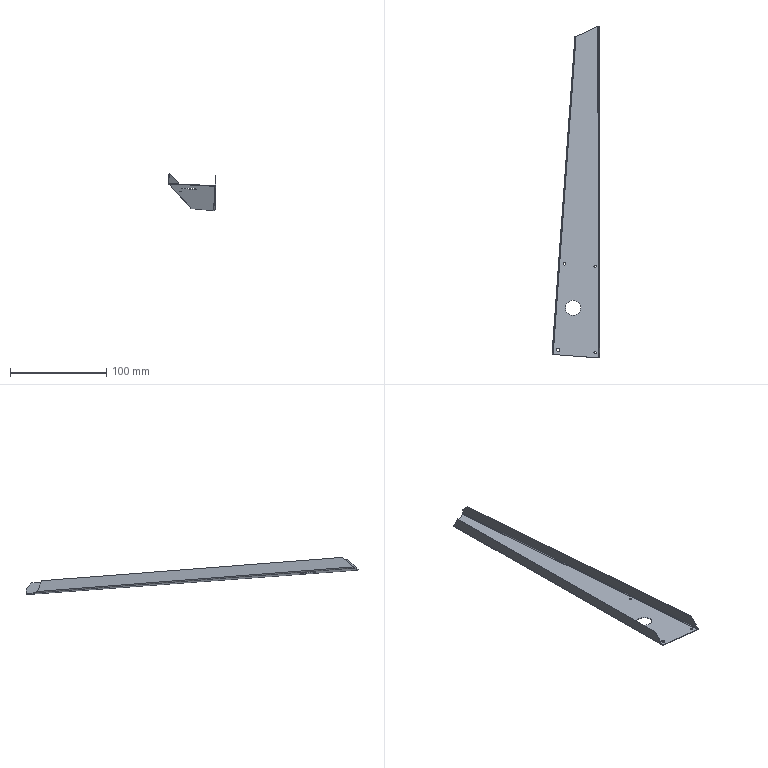Part | SolidWorks | features BaseBody 1 | 1 solid | 37 faces | box 49.869 x 345.626 x 38.793 mm | volume 9891 mm3 | cylinder 16 | plane 15 | spline 6 | commonest cylinder face diameters 2.4 x6 1.473 x3 2.473 x3 3.385 x2 15.9 x2
STEP:
#1=CARTESIAN_POINT('',(-25.934,44.235,46.553));
#2=VERTEX_POINT('',#1);
#3=CARTESIAN_POINT('',(-25.934,60.092,45.382));
#4=VERTEX_POINT('',#3);
#5=CARTESIAN_POINT('',(-25.934,52.163,45.968));
#6=DIRECTION('',(-0.05227,-0.07356,-0.9959));
#7=DIRECTION('',(0.,-0.9973,0.07366));
#8=AXIS2_PLACEMENT_3D('',#5,#6,#7);
#9=CIRCLE('',#8,7.95);
#10=EDGE_CURVE('',#2,#4,#9,.T.);
#11=ORIENTED_EDGE('',*,*,#10,.T.);
#12=CARTESIAN_POINT('',(-25.908,60.128,45.88));
#13=VERTEX_POINT('',#12);
#14=CARTESIAN_POINT('',(-25.934,60.092,45.382));
#15=DIRECTION('',(0.05227,0.07356,0.9959));
#16=VECTOR('',#15,1000.);
#17=LINE('',#14,#16);
#18=EDGE_CURVE('',#4,#13,#17,.T.);
#19=ORIENTED_EDGE('',*,*,#18,.T.);
#20=CARTESIAN_POINT('',(-25.908,44.272,47.051));
#21=VERTEX_POINT('',#20);
#22=CARTESIAN_POINT('',(-25.908,52.2,46.466));
#23=DIRECTION('',(0.05227,0.07356,0.9959));
#24=DIRECTION('',(0.,-0.9973,0.07366));
#25=AXIS2_PLACEMENT_3D('',#22,#23,#24);
#26=CIRCLE('',#25,7.95);
#27=EDGE_CURVE('',#13,#21,#26,.T.);
#28=ORIENTED_EDGE('',*,*,#27,.T.);
#29=CARTESIAN_POINT('',(-25.934,44.235,46.553));
#30=DIRECTION('',(0.05227,0.07356,0.9959));
#31=VECTOR('',#30,1000.);
#32=LINE('',#29,#31);
#33=EDGE_CURVE('',#2,#21,#32,.T.);
#34=ORIENTED_EDGE('',*,*,#33,.F.);
#35=EDGE_LOOP('',(#11,#19,#28,#34));
#36=FACE_OUTER_BOUND('',#35,.T.);
#37=CARTESIAN_POINT('',(-25.934,52.163,45.968));
#38=DIRECTION('',(0.05227,0.07356,0.9959));
#39=DIRECTION('',(0.,-0.9973,0.07366));
#40=AXIS2_PLACEMENT_3D('',#37,#38,#39);
#41=CYLINDRICAL_SURFACE('',#40,7.95);
#42=ADVANCED_FACE('',(#36),#41,.F.);
#43=CARTESIAN_POINT('',(-3.009,96.582,41.484));
#44=VERTEX_POINT('',#43);
#45=CARTESIAN_POINT('',(-3.009,94.189,41.661));
#46=VERTEX_POINT('',#45);
#47=CARTESIAN_POINT('',(-3.009,95.385,41.572));
#48=DIRECTION('',(0.05227,0.07356,0.9959));
#49=DIRECTION('',(0.,-0.9973,0.07366));
#50=AXIS2_PLACEMENT_3D('',#47,#48,#49);
#51=CIRCLE('',#50,1.2);
#52=EDGE_CURVE('',#44,#46,#51,.T.);
#53=ORIENTED_EDGE('',*,*,#52,.F.);
#54=CARTESIAN_POINT('',(-2.982,96.619,41.982));
#55=VERTEX_POINT('',#54);
#56=CARTESIAN_POINT('',(-3.009,96.582,41.484));
#57=DIRECTION('',(0.05227,0.07356,0.9959));
#58=VECTOR('',#57,1000.);
#59=LINE('',#56,#58);
#60=EDGE_CURVE('',#44,#55,#59,.T.);
#61=ORIENTED_EDGE('',*,*,#60,.T.);
#62=CARTESIAN_POINT('',(-2.982,94.225,42.159));
#63=VERTEX_POINT('',#62);
#64=CARTESIAN_POINT('',(-2.982,95.422,42.07));
#65=DIRECTION('',(0.05227,0.07356,0.9959));
#66=DIRECTION('',(0.,-0.9973,0.07366));
#67=AXIS2_PLACEMENT_3D('',#64,#65,#66);
#68=CIRCLE('',#67,1.2);
#69=EDGE_CURVE('',#55,#63,#68,.T.);
#70=ORIENTED_EDGE('',*,*,#69,.T.);
#71=CARTESIAN_POINT('',(-3.009,94.189,41.661));
#72=DIRECTION('',(0.05227,0.07356,0.9959));
#73=VECTOR('',#72,1000.);
#74=LINE('',#71,#73);
#75=EDGE_CURVE('',#46,#63,#74,.T.);
#76=ORIENTED_EDGE('',*,*,#75,.F.);
#77=EDGE_LOOP('',(#53,#61,#70,#76));
#78=FACE_OUTER_BOUND('',#77,.T.);
#79=CARTESIAN_POINT('',(-3.009,95.385,41.572));
#80=DIRECTION('',(0.05227,0.07356,0.9959));
#81=DIRECTION('',(0.,-0.9973,0.07366));
#82=AXIS2_PLACEMENT_3D('',#79,#80,#81);
#83=CYLINDRICAL_SURFACE('',#82,1.2);
#84=ADVANCED_FACE('',(#78),#83,.F.);
#85=CARTESIAN_POINT('',(-34.851,99.051,42.973));
#86=VERTEX_POINT('',#85);
#87=CARTESIAN_POINT('',(-34.851,96.658,43.149));
#88=VERTEX_POINT('',#87);
#89=CARTESIAN_POINT('',(-34.851,97.854,43.061));
#90=DIRECTION('',(0.05227,0.07356,0.9959));
#91=DIRECTION('',(0.,-0.9973,0.07366));
#92=AXIS2_PLACEMENT_3D('',#89,#90,#91);
#93=CIRCLE('',#92,1.2);
#94=EDGE_CURVE('',#86,#88,#93,.T.);
#95=ORIENTED_EDGE('',*,*,#94,.F.);
#96=CARTESIAN_POINT('',(-34.825,99.088,43.471));
#97=VERTEX_POINT('',#96);
#98=CARTESIAN_POINT('',(-34.851,99.051,42.973));
#99=DIRECTION('',(0.05227,0.07356,0.9959));
#100=VECTOR('',#99,1000.);
#101=LINE('',#98,#100);
#102=EDGE_CURVE('',#86,#97,#101,.T.);
#103=ORIENTED_EDGE('',*,*,#102,.T.);
#104=CARTESIAN_POINT('',(-34.825,96.694,43.647));
#105=VERTEX_POINT('',#104);
#106=CARTESIAN_POINT('',(-34.825,97.891,43.559));
#107=DIRECTION('',(0.05227,0.07356,0.9959));
#108=DIRECTION('',(0.,-0.9973,0.07366));
#109=AXIS2_PLACEMENT_3D('',#106,#107,#108);
#110=CIRCLE('',#109,1.2);
#111=EDGE_CURVE('',#97,#105,#110,.T.);
#112=ORIENTED_EDGE('',*,*,#111,.T.);
#113=CARTESIAN_POINT('',(-34.851,96.658,43.149));
#114=DIRECTION('',(0.05227,0.07356,0.9959));
#115=VECTOR('',#114,1000.);
#116=LINE('',#113,#115);
#117=EDGE_CURVE('',#88,#105,#116,.T.);
#118=ORIENTED_EDGE('',*,*,#117,.F.);
#119=EDGE_LOOP('',(#95,#103,#112,#118));
#120=FACE_OUTER_BOUND('',#119,.T.);
#121=CARTESIAN_POINT('',(-34.851,97.854,43.061));
#122=DIRECTION('',(0.05227,0.07356,0.9959));
#123=DIRECTION('',(0.,-0.9973,0.07366));
#124=AXIS2_PLACEMENT_3D('',#121,#122,#123);
#125=CYLINDRICAL_SURFACE('',#124,1.2);
#126=ADVANCED_FACE('',(#120),#125,.F.);
#127=CARTESIAN_POINT('',(-3.008,6.583,48.131));
#128=VERTEX_POINT('',#127);
#129=CARTESIAN_POINT('',(-3.008,4.189,48.308));
#130=VERTEX_POINT('',#129);
#131=CARTESIAN_POINT('',(-3.008,5.386,48.22));
#132=DIRECTION('',(0.05227,0.07356,0.9959));
#133=DIRECTION('',(0.,-0.9973,0.07366));
#134=AXIS2_PLACEMENT_3D('',#131,#132,#133);
#135=CIRCLE('',#134,1.2);
#136=EDGE_CURVE('',#128,#130,#135,.T.);
#137=ORIENTED_EDGE('',*,*,#136,.F.);
#138=CARTESIAN_POINT('',(-2.982,6.619,48.629));
#139=VERTEX_POINT('',#138);
#140=CARTESIAN_POINT('',(-3.008,6.583,48.131));
#141=DIRECTION('',(0.05227,0.07356,0.9959));
#142=VECTOR('',#141,1000.);
#143=LINE('',#140,#142);
#144=EDGE_CURVE('',#128,#139,#143,.T.);
#145=ORIENTED_EDGE('',*,*,#144,.T.);
#146=CARTESIAN_POINT('',(-2.982,4.226,48.806));
#147=VERTEX_POINT('',#146);
#148=CARTESIAN_POINT('',(-2.982,5.423,48.718));
#149=DIRECTION('',(0.05227,0.07356,0.9959));
#150=DIRECTION('',(0.,-0.9973,0.07366));
#151=AXIS2_PLACEMENT_3D('',#148,#149,#150);
#152=CIRCLE('',#151,1.2);
#153=EDGE_CURVE('',#139,#147,#152,.T.);
#154=ORIENTED_EDGE('',*,*,#153,.T.);
#155=CARTESIAN_POINT('',(-3.008,4.189,48.308));
#156=DIRECTION('',(0.05227,0.07356,0.9959));
#157=VECTOR('',#156,1000.);
#158=LINE('',#155,#157);
#159=EDGE_CURVE('',#130,#147,#158,.T.);
#160=ORIENTED_EDGE('',*,*,#159,.F.);
#161=EDGE_LOOP('',(#137,#145,#154,#160));
#162=FACE_OUTER_BOUND('',#161,.T.);
#163=CARTESIAN_POINT('',(-3.008,5.386,48.22));
#164=DIRECTION('',(0.05227,0.07356,0.9959));
#165=DIRECTION('',(0.,-0.9973,0.07366));
#166=AXIS2_PLACEMENT_3D('',#163,#164,#165);
#167=CYLINDRICAL_SURFACE('',#166,1.2);
#168=ADVANCED_FACE('',(#162),#167,.F.);
#169=CARTESIAN_POINT('',(-41.464,10.056,49.893));
#170=VERTEX_POINT('',#169);
#171=CARTESIAN_POINT('',(-41.464,6.68,50.142));
#172=VERTEX_POINT('',#171);
#173=CARTESIAN_POINT('',(-41.464,8.368,50.018));
#174=DIRECTION('',(0.05227,0.07356,0.9959));
#175=DIRECTION('',(0.,-0.9973,0.07366));
#176=AXIS2_PLACEMENT_3D('',#173,#174,#175);
#177=CIRCLE('',#176,1.693);
#178=EDGE_CURVE('',#170,#172,#177,.T.);
#179=ORIENTED_EDGE('',*,*,#178,.F.);
#180=CARTESIAN_POINT('',(-41.438,10.092,50.391));
#181=VERTEX_POINT('',#180);
#182=CARTESIAN_POINT('',(-41.464,10.056,49.893));
#183=DIRECTION('',(0.05227,0.07356,0.9959));
#184=VECTOR('',#183,1000.);
#185=LINE('',#182,#184);
#186=EDGE_CURVE('',#170,#181,#185,.T.);
#187=ORIENTED_EDGE('',*,*,#186,.T.);
#188=CARTESIAN_POINT('',(-41.438,6.716,50.64));
#189=VERTEX_POINT('',#188);
#190=CARTESIAN_POINT('',(-41.438,8.404,50.516));
#191=DIRECTION('',(0.05227,0.07356,0.9959));
#192=DIRECTION('',(0.,-0.9973,0.07366));
#193=AXIS2_PLACEMENT_3D('',#190,#191,#192);
#194=CIRCLE('',#193,1.693);
#195=EDGE_CURVE('',#181,#189,#194,.T.);
#196=ORIENTED_EDGE('',*,*,#195,.T.);
#197=CARTESIAN_POINT('',(-41.464,6.68,50.142));
#198=DIRECTION('',(0.05227,0.07356,0.9959));
#199=VECTOR('',#198,1000.);
#200=LINE('',#197,#199);
#201=EDGE_CURVE('',#172,#189,#200,.T.);
#202=ORIENTED_EDGE('',*,*,#201,.F.);
#203=EDGE_LOOP('',(#179,#187,#196,#202));
#204=FACE_OUTER_BOUND('',#203,.T.);
#205=CARTESIAN_POINT('',(-41.464,8.368,50.018));
#206=DIRECTION('',(0.05227,0.07356,0.9959));
#207=DIRECTION('',(0.,-0.9973,0.07366));
#208=AXIS2_PLACEMENT_3D('',#205,#206,#207);
#209=CYLINDRICAL_SURFACE('',#208,1.693);
#210=ADVANCED_FACE('',(#204),#209,.F.);
#211=CARTESIAN_POINT('',(0.4134,345.618,23.653));
#212=VERTEX_POINT('',#211);
#213=CARTESIAN_POINT('',(-0.1031,345.249,23.468));
#214=VERTEX_POINT('',#213);
#215=CARTESIAN_POINT('',(0.4134,345.618,23.653));
#216=CARTESIAN_POINT('',(0.345,345.554,23.59));
#217=CARTESIAN_POINT('',(0.2656,345.492,23.542));
#218=CARTESIAN_POINT('',(0.08824,345.368,23.478));
#219=CARTESIAN_POINT('',(-0.007361,345.308,23.463));
#220=CARTESIAN_POINT('',(-0.1031,345.249,23.468));
#221=B_SPLINE_CURVE_WITH_KNOTS('',3,(#215,#216,#217,#218,#219,#220),.UNSPECIFIED.,.F.,.F.,(4,2,4),(0.,0.0003341,0.0006683),.UNSPECIFIED.);
#222=EDGE_CURVE('',#212,#214,#221,.T.);
#223=ORIENTED_EDGE('',*,*,#222,.T.);
#224=CARTESIAN_POINT('',(0.5636,0.05796,48.929));
#225=VERTEX_POINT('',#224);
#226=CARTESIAN_POINT('',(-0.1078,347.675,23.289));
#227=DIRECTION('',(0.001926,-0.9973,0.07356));
#228=VECTOR('',#227,1000.);
#229=LINE('',#226,#228);
#230=EDGE_CURVE('',#214,#225,#229,.T.);
#231=ORIENTED_EDGE('',*,*,#230,.T.);
#232=CARTESIAN_POINT('',(1.081,0.01805,49.144));
#233=VERTEX_POINT('',#232);
#234=CARTESIAN_POINT('',(0.5636,0.05796,48.929));
#235=CARTESIAN_POINT('',(0.7548,0.03949,48.93));
#236=CARTESIAN_POINT('',(0.9448,0.02675,49.009));
#237=CARTESIAN_POINT('',(1.081,0.01805,49.144));
#238=B_SPLINE_CURVE_WITH_KNOTS('',3,(#234,#235,#236,#237),.UNSPECIFIED.,.F.,.F.,(4,4),(0.06296,1.),.UNSPECIFIED.);
#239=EDGE_CURVE('',#225,#233,#238,.T.);
#240=ORIENTED_EDGE('',*,*,#239,.T.);
#241=CARTESIAN_POINT('',(1.299,0.7061,49.6));
#242=VERTEX_POINT('',#241);
#243=CARTESIAN_POINT('',(1.081,0.01805,49.144));
#244=CARTESIAN_POINT('',(1.215,0.2454,49.26));
#245=CARTESIAN_POINT('',(1.294,0.4748,49.428));
#246=CARTESIAN_POINT('',(1.299,0.7061,49.6));
#247=B_SPLINE_CURVE_WITH_KNOTS('',3,(#243,#244,#245,#246),.UNSPECIFIED.,.F.,.F.,(4,4),(0.,0.0008625),.UNSPECIFIED.);
#248=EDGE_CURVE('',#233,#242,#247,.T.);
#249=ORIENTED_EDGE('',*,*,#248,.T.);
#250=CARTESIAN_POINT('',(0.6327,345.6,24.161));
#251=VERTEX_POINT('',#250);
#252=CARTESIAN_POINT('',(0.9663,172.856,36.903));
#253=DIRECTION('',(-0.001926,0.9973,-0.07356));
#254=VECTOR('',#253,1000.);
#255=LINE('',#252,#254);
#256=EDGE_CURVE('',#242,#251,#255,.T.);
#257=ORIENTED_EDGE('',*,*,#256,.T.);
#258=CARTESIAN_POINT('',(0.6327,345.6,24.161));
#259=CARTESIAN_POINT('',(0.6277,345.605,23.972));
#260=CARTESIAN_POINT('',(0.5474,345.609,23.786));
#261=CARTESIAN_POINT('',(0.4134,345.618,23.653));
#262=B_SPLINE_CURVE_WITH_KNOTS('',3,(#258,#259,#260,#261),.UNSPECIFIED.,.F.,.F.,(4,4),(0.,1.),.UNSPECIFIED.);
#263=EDGE_CURVE('',#251,#212,#262,.T.);
#264=ORIENTED_EDGE('',*,*,#263,.T.);
#265=EDGE_LOOP('',(#223,#231,#240,#249,#257,#264));
#266=FACE_OUTER_BOUND('',#265,.T.);
#267=CARTESIAN_POINT('',(-0.1078,347.729,24.023));
#268=DIRECTION('',(0.001926,-0.9973,0.07356));
#269=DIRECTION('',(0.,-0.07356,-0.9973));
#270=AXIS2_PLACEMENT_3D('',#267,#268,#269);
#271=CYLINDRICAL_SURFACE('',#270,0.7366);
#272=ADVANCED_FACE('',(#266),#271,.F.);
#273=CARTESIAN_POINT('',(-0.1031,345.212,22.969));
#274=VERTEX_POINT('',#273);
#275=CARTESIAN_POINT('',(-0.1677,345.188,22.973));
#276=VERTEX_POINT('',#275);
#277=CARTESIAN_POINT('',(-0.1031,345.212,22.969));
#278=CARTESIAN_POINT('',(-0.1246,345.204,22.97));
#279=CARTESIAN_POINT('',(-0.1461,345.196,22.971));
#280=CARTESIAN_POINT('',(-0.1677,345.188,22.973));
#281=B_SPLINE_CURVE_WITH_KNOTS('',3,(#277,#278,#279,#280),.UNSPECIFIED.,.F.,.F.,(4,4),(0.00102,0.001088),.UNSPECIFIED.);
#282=EDGE_CURVE('',#274,#276,#281,.T.);
#283=ORIENTED_EDGE('',*,*,#282,.F.);
#284=CARTESIAN_POINT('',(0.5636,0.02118,48.43));
#285=VERTEX_POINT('',#284);
#286=CARTESIAN_POINT('',(-0.1078,347.638,22.79));
#287=DIRECTION('',(0.001926,-0.9973,0.07356));
#288=VECTOR('',#287,1000.);
#289=LINE('',#286,#288);
#290=EDGE_CURVE('',#274,#285,#289,.T.);
#291=ORIENTED_EDGE('',*,*,#290,.T.);
#292=CARTESIAN_POINT('',(0.499,0.02497,48.432));
#293=VERTEX_POINT('',#292);
#294=CARTESIAN_POINT('',(0.499,0.02497,48.432));
#295=CARTESIAN_POINT('',(0.5205,0.02367,48.431));
#296=CARTESIAN_POINT('',(0.5421,0.0224,48.43));
#297=CARTESIAN_POINT('',(0.5636,0.02118,48.43));
#298=B_SPLINE_CURVE_WITH_KNOTS('',3,(#294,#295,#296,#297),.UNSPECIFIED.,.F.,.F.,(4,4),(0.,0.06296),.UNSPECIFIED.);
#299=EDGE_CURVE('',#293,#285,#298,.T.);
#300=ORIENTED_EDGE('',*,*,#299,.F.);
#301=CARTESIAN_POINT('',(-0.1677,345.188,22.973));
#302=DIRECTION('',(0.001926,-0.9973,0.07356));
#303=VECTOR('',#302,1000.);
#304=LINE('',#301,#303);
#305=EDGE_CURVE('',#276,#293,#304,.T.);
#306=ORIENTED_EDGE('',*,*,#305,.F.);
#307=EDGE_LOOP('',(#283,#291,#300,#306));
#308=FACE_OUTER_BOUND('',#307,.T.);
#309=CARTESIAN_POINT('',(-0.1078,347.729,24.023));
#310=DIRECTION('',(0.001926,-0.9973,0.07356));
#311=DIRECTION('',(0.,-0.07356,-0.9973));
#312=AXIS2_PLACEMENT_3D('',#309,#310,#311);
#313=CYLINDRICAL_SURFACE('',#312,1.237);
#314=ADVANCED_FACE('',(#308),#313,.T.);
#315=ORIENTED_EDGE('',*,*,#18,.F.);
#316=CARTESIAN_POINT('',(-25.934,52.163,45.968));
#317=DIRECTION('',(-0.05227,-0.07356,-0.9959));
#318=DIRECTION('',(0.,-0.9973,0.07366));
#319=AXIS2_PLACEMENT_3D('',#316,#317,#318);
#320=CIRCLE('',#319,7.95);
#321=EDGE_CURVE('',#4,#2,#320,.T.);
#322=ORIENTED_EDGE('',*,*,#321,.T.);
#323=ORIENTED_EDGE('',*,*,#33,.T.);
#324=CARTESIAN_POINT('',(-25.908,52.2,46.466));
#325=DIRECTION('',(0.05227,0.07356,0.9959));
#326=DIRECTION('',(0.,-0.9973,0.07366));
#327=AXIS2_PLACEMENT_3D('',#324,#325,#326);
#328=CIRCLE('',#327,7.95);
#329=EDGE_CURVE('',#21,#13,#328,.T.);
#330=ORIENTED_EDGE('',*,*,#329,.T.);
#331=EDGE_LOOP('',(#315,#322,#323,#330));
#332=FACE_OUTER_BOUND('',#331,.T.);
#333=CARTESIAN_POINT('',(-25.934,52.163,45.968));
#334=DIRECTION('',(0.05227,0.07356,0.9959));
#335=DIRECTION('',(0.,-0.9973,0.07366));
#336=AXIS2_PLACEMENT_3D('',#333,#334,#335);
#337=CYLINDRICAL_SURFACE('',#336,7.95);
#338=ADVANCED_FACE('',(#332),#337,.F.);
#339=CARTESIAN_POINT('',(-2.982,95.422,42.07));
#340=DIRECTION('',(0.05227,0.07356,0.9959));
#341=DIRECTION('',(0.,-0.9973,0.07366));
#342=AXIS2_PLACEMENT_3D('',#339,#340,#341);
#343=CIRCLE('',#342,1.2);
#344=EDGE_CURVE('',#63,#55,#343,.T.);
#345=ORIENTED_EDGE('',*,*,#344,.F.);
#346=ORIENTED_EDGE('',*,*,#69,.F.);
#347=EDGE_LOOP('',(#345,#346));
#348=FACE_BOUND('',#347,.T.);
#349=CARTESIAN_POINT('',(-34.825,97.891,43.559));
#350=DIRECTION('',(0.05227,0.07356,0.9959));
#351=DIRECTION('',(0.,-0.9973,0.07366));
#352=AXIS2_PLACEMENT_3D('',#349,#350,#351);
#353=CIRCLE('',#352,1.2);
#354=EDGE_CURVE('',#105,#97,#353,.T.);
#355=ORIENTED_EDGE('',*,*,#354,.F.);
#356=ORIENTED_EDGE('',*,*,#111,.F.);
#357=EDGE_LOOP('',(#355,#356));
#358=FACE_BOUND('',#357,.T.);
#359=CARTESIAN_POINT('',(-2.982,5.423,48.718));
#360=DIRECTION('',(0.05227,0.07356,0.9959));
#361=DIRECTION('',(0.,-0.9973,0.07366));
#362=AXIS2_PLACEMENT_3D('',#359,#360,#361);
#363=CIRCLE('',#362,1.2);
#364=EDGE_CURVE('',#147,#139,#363,.T.);
#365=ORIENTED_EDGE('',*,*,#364,.F.);
#366=ORIENTED_EDGE('',*,*,#153,.F.);
#367=EDGE_LOOP('',(#365,#366));
#368=FACE_BOUND('',#367,.T.);
#369=CARTESIAN_POINT('',(-41.438,8.404,50.516));
#370=DIRECTION('',(0.05227,0.07356,0.9959));
#371=DIRECTION('',(0.,-0.9973,0.07366));
#372=AXIS2_PLACEMENT_3D('',#369,#370,#371);
#373=CIRCLE('',#372,1.693);
#374=EDGE_CURVE('',#189,#181,#373,.T.);
#375=ORIENTED_EDGE('',*,*,#374,.F.);
#376=ORIENTED_EDGE('',*,*,#195,.F.);
#377=EDGE_LOOP('',(#375,#376));
#378=FACE_BOUND('',#377,.T.);
#379=ORIENTED_EDGE('',*,*,#329,.F.);
#380=ORIENTED_EDGE('',*,*,#27,.F.);
#381=EDGE_LOOP('',(#379,#380));
#382=FACE_BOUND('',#381,.T.);
#383=CARTESIAN_POINT('',(-46.66,3.629,51.142));
#384=VERTEX_POINT('',#383);
#385=CARTESIAN_POINT('',(-22.827,334.825,25.429));
#386=VERTEX_POINT('',#385);
#387=CARTESIAN_POINT('',(-34.236,176.282,37.738));
#388=DIRECTION('',(0.07156,0.9944,-0.07721));
#389=VECTOR('',#388,1000.);
#390=LINE('',#387,#389);
#391=EDGE_CURVE('',#384,#386,#390,.T.);
#392=ORIENTED_EDGE('',*,*,#391,.F.);
#393=CARTESIAN_POINT('',(0.5251,0.06175,48.93));
#394=VERTEX_POINT('',#393);
#395=CARTESIAN_POINT('',(-22.926,1.835,50.029));
#396=DIRECTION('',(-0.9961,0.07531,0.04671));
#397=VECTOR('',#396,1000.);
#398=LINE('',#395,#397);
#399=EDGE_CURVE('',#394,#384,#398,.T.);
#400=ORIENTED_EDGE('',*,*,#399,.F.);
#401=CARTESIAN_POINT('',(-0.1415,345.225,23.47));
#402=VERTEX_POINT('',#401);
#403=CARTESIAN_POINT('',(-0.1463,347.675,23.29));
#404=DIRECTION('',(0.001926,-0.9973,0.07356));
#405=VECTOR('',#404,1000.);
#406=LINE('',#403,#405);
#407=EDGE_CURVE('',#402,#394,#406,.T.);
#408=ORIENTED_EDGE('',*,*,#407,.F.);
#409=CARTESIAN_POINT('',(-22.827,334.825,25.429));
#410=DIRECTION('',(0.9062,0.4155,-0.07825));
#411=VECTOR('',#410,1000.);
#412=LINE('',#409,#411);
#413=EDGE_CURVE('',#386,#402,#412,.T.);
#414=ORIENTED_EDGE('',*,*,#413,.F.);
#415=EDGE_LOOP('',(#392,#400,#408,#414));
#416=FACE_OUTER_BOUND('',#415,.T.);
#417=CARTESIAN_POINT('',(-21.811,348.934,24.334));
#418=DIRECTION('',(-0.05227,-0.07356,-0.9959));
#419=DIRECTION('',(0.9961,-0.07531,-0.04671));
#420=AXIS2_PLACEMENT_3D('',#417,#418,#419);
#421=PLANE('',#420);
#422=ADVANCED_FACE('',(#348,#358,#368,#378,#382,#416),#421,.F.);
#423=CARTESIAN_POINT('',(-3.009,95.385,41.572));
#424=DIRECTION('',(0.05227,0.07356,0.9959));
#425=DIRECTION('',(0.,-0.9973,0.07366));
#426=AXIS2_PLACEMENT_3D('',#423,#424,#425);
#427=CIRCLE('',#426,1.2);
#428=EDGE_CURVE('',#46,#44,#427,.T.);
#429=ORIENTED_EDGE('',*,*,#428,.T.);
#430=ORIENTED_EDGE('',*,*,#52,.T.);
#431=EDGE_LOOP('',(#429,#430));
#432=FACE_BOUND('',#431,.T.);
#433=CARTESIAN_POINT('',(-34.851,97.854,43.061));
#434=DIRECTION('',(0.05227,0.07356,0.9959));
#435=DIRECTION('',(0.,-0.9973,0.07366));
#436=AXIS2_PLACEMENT_3D('',#433,#434,#435);
#437=CIRCLE('',#436,1.2);
#438=EDGE_CURVE('',#88,#86,#437,.T.);
#439=ORIENTED_EDGE('',*,*,#438,.T.);
#440=ORIENTED_EDGE('',*,*,#94,.T.);
#441=EDGE_LOOP('',(#439,#440));
#442=FACE_BOUND('',#441,.T.);
#443=CARTESIAN_POINT('',(-3.008,5.386,48.22));
#444=DIRECTION('',(0.05227,0.07356,0.9959));
#445=DIRECTION('',(0.,-0.9973,0.07366));
#446=AXIS2_PLACEMENT_3D('',#443,#444,#445);
#447=CIRCLE('',#446,1.2);
#448=EDGE_CURVE('',#130,#128,#447,.T.);
#449=ORIENTED_EDGE('',*,*,#448,.T.);
#450=ORIENTED_EDGE('',*,*,#136,.T.);
#451=EDGE_LOOP('',(#449,#450));
#452=FACE_BOUND('',#451,.T.);
#453=CARTESIAN_POINT('',(-41.464,8.368,50.018));
#454=DIRECTION('',(0.05227,0.07356,0.9959));
#455=DIRECTION('',(0.,-0.9973,0.07366));
#456=AXIS2_PLACEMENT_3D('',#453,#454,#455);
#457=CIRCLE('',#456,1.693);
#458=EDGE_CURVE('',#172,#170,#457,.T.);
#459=ORIENTED_EDGE('',*,*,#458,.T.);
#460=ORIENTED_EDGE('',*,*,#178,.T.);
#461=EDGE_LOOP('',(#459,#460));
#462=FACE_BOUND('',#461,.T.);
#463=ORIENTED_EDGE('',*,*,#10,.F.);
#464=ORIENTED_EDGE('',*,*,#321,.F.);
#465=EDGE_LOOP('',(#463,#464));
#466=FACE_BOUND('',#465,.T.);
#467=CARTESIAN_POINT('',(-46.687,3.592,50.644));
#468=VERTEX_POINT('',#467);
#469=CARTESIAN_POINT('',(-22.853,334.788,24.931));
#470=VERTEX_POINT('',#469);
#471=CARTESIAN_POINT('',(-34.262,176.245,37.24));
#472=DIRECTION('',(0.07156,0.9944,-0.07721));
#473=VECTOR('',#472,1000.);
#474=LINE('',#471,#473);
#475=EDGE_CURVE('',#468,#470,#474,.T.);
#476=ORIENTED_EDGE('',*,*,#475,.T.);
#477=CARTESIAN_POINT('',(-22.853,334.788,24.931));
#478=DIRECTION('',(0.9062,0.4155,-0.07825));
#479=VECTOR('',#478,1000.);
#480=LINE('',#477,#479);
#481=EDGE_CURVE('',#470,#276,#480,.T.);
#482=ORIENTED_EDGE('',*,*,#481,.T.);
#483=ORIENTED_EDGE('',*,*,#305,.T.);
#484=CARTESIAN_POINT('',(-22.952,1.798,49.531));
#485=DIRECTION('',(-0.9961,0.07531,0.04671));
#486=VECTOR('',#485,1000.);
#487=LINE('',#484,#486);
#488=EDGE_CURVE('',#293,#468,#487,.T.);
#489=ORIENTED_EDGE('',*,*,#488,.T.);
#490=EDGE_LOOP('',(#476,#482,#483,#489));
#491=FACE_OUTER_BOUND('',#490,.T.);
#492=CARTESIAN_POINT('',(-21.838,348.897,23.836));
#493=DIRECTION('',(-0.05227,-0.07356,-0.9959));
#494=DIRECTION('',(0.9961,-0.07531,-0.04671));
#495=AXIS2_PLACEMENT_3D('',#492,#493,#494);
#496=PLANE('',#495);
#497=ADVANCED_FACE('',(#432,#442,#452,#462,#466,#491),#496,.T.);
#498=ORIENTED_EDGE('',*,*,#60,.F.);
#499=ORIENTED_EDGE('',*,*,#428,.F.);
#500=ORIENTED_EDGE('',*,*,#75,.T.);
#501=ORIENTED_EDGE('',*,*,#344,.T.);
#502=EDGE_LOOP('',(#498,#499,#500,#501));
#503=FACE_OUTER_BOUND('',#502,.T.);
#504=CARTESIAN_POINT('',(-3.009,95.385,41.572));
#505=DIRECTION('',(0.05227,0.07356,0.9959));
#506=DIRECTION('',(0.,-0.9973,0.07366));
#507=AXIS2_PLACEMENT_3D('',#504,#505,#506);
#508=CYLINDRICAL_SURFACE('',#507,1.2);
#509=ADVANCED_FACE('',(#503),#508,.F.);
#510=ORIENTED_EDGE('',*,*,#102,.F.);
#511=ORIENTED_EDGE('',*,*,#438,.F.);
#512=ORIENTED_EDGE('',*,*,#117,.T.);
#513=ORIENTED_EDGE('',*,*,#354,.T.);
#514=EDGE_LOOP('',(#510,#511,#512,#513));
#515=FACE_OUTER_BOUND('',#514,.T.);
#516=CARTESIAN_POINT('',(-34.851,97.854,43.061));
#517=DIRECTION('',(0.05227,0.07356,0.9959));
#518=DIRECTION('',(0.,-0.9973,0.07366));
#519=AXIS2_PLACEMENT_3D('',#516,#517,#518);
#520=CYLINDRICAL_SURFACE('',#519,1.2);
#521=ADVANCED_FACE('',(#515),#520,.F.);
#522=ORIENTED_EDGE('',*,*,#144,.F.);
#523=ORIENTED_EDGE('',*,*,#448,.F.);
#524=ORIENTED_EDGE('',*,*,#159,.T.);
#525=ORIENTED_EDGE('',*,*,#364,.T.);
#526=EDGE_LOOP('',(#522,#523,#524,#525));
#527=FACE_OUTER_BOUND('',#526,.T.);
#528=CARTESIAN_POINT('',(-3.008,5.386,48.22));
#529=DIRECTION('',(0.05227,0.07356,0.9959));
#530=DIRECTION('',(0.,-0.9973,0.07366));
#531=AXIS2_PLACEMENT_3D('',#528,#529,#530);
#532=CYLINDRICAL_SURFACE('',#531,1.2);
#533=ADVANCED_FACE('',(#527),#532,.F.);
#534=ORIENTED_EDGE('',*,*,#186,.F.);
#535=ORIENTED_EDGE('',*,*,#458,.F.);
#536=ORIENTED_EDGE('',*,*,#201,.T.);
#537=ORIENTED_EDGE('',*,*,#374,.T.);
#538=EDGE_LOOP('',(#534,#535,#536,#537));
#539=FACE_OUTER_BOUND('',#538,.T.);
#540=CARTESIAN_POINT('',(-41.464,8.368,50.018));
#541=DIRECTION('',(0.05227,0.07356,0.9959));
#542=DIRECTION('',(0.,-0.9973,0.07366));
#543=AXIS2_PLACEMENT_3D('',#540,#541,#542);
#544=CYLINDRICAL_SURFACE('',#543,1.693);
#545=ADVANCED_FACE('',(#539),#544,.F.);
#546=CARTESIAN_POINT('',(-22.84,334.806,25.18));
#547=DIRECTION('',(0.05227,0.07356,0.9959));
#548=VECTOR('',#547,1000.);
#549=LINE('',#546,#548);
#550=EDGE_CURVE('',#470,#386,#549,.T.);
#551=ORIENTED_EDGE('',*,*,#550,.T.);
#552=ORIENTED_EDGE('',*,*,#413,.T.);
#553=CARTESIAN_POINT('',(-0.1546,345.207,23.221));
#554=DIRECTION('',(0.05227,0.07356,0.9959));
#555=VECTOR('',#554,1000.);
#556=LINE('',#553,#555);
#557=EDGE_CURVE('',#276,#402,#556,.T.);
#558=ORIENTED_EDGE('',*,*,#557,.F.);
#559=ORIENTED_EDGE('',*,*,#481,.F.);
#560=EDGE_LOOP('',(#551,#552,#558,#559));
#561=FACE_OUTER_BOUND('',#560,.T.);
#562=CARTESIAN_POINT('',(-22.853,334.788,24.931));
#563=DIRECTION('',(0.4195,-0.9066,0.04495));
#564=DIRECTION('',(0.9062,0.4155,-0.07825));
#565=AXIS2_PLACEMENT_3D('',#562,#563,#564);
#566=PLANE('',#565);
#567=ADVANCED_FACE('',(#561),#566,.F.);
#568=CARTESIAN_POINT('',(-23.583,334.095,26.243));
#569=VERTEX_POINT('',#568);
#570=CARTESIAN_POINT('',(-22.827,334.825,25.429));
#571=CARTESIAN_POINT('',(-22.927,334.761,25.439));
#572=CARTESIAN_POINT('',(-23.024,334.701,25.467));
#573=CARTESIAN_POINT('',(-23.206,334.579,25.557));
#574=CARTESIAN_POINT('',(-23.288,334.52,25.619));
#575=CARTESIAN_POINT('',(-23.496,334.34,25.842));
#576=CARTESIAN_POINT('',(-23.578,334.221,26.041));
#577=CARTESIAN_POINT('',(-23.583,334.095,26.243));
#578=B_SPLINE_CURVE_WITH_KNOTS('',3,(#570,#571,#572,#573,#574,#575,#576,#577),.UNSPECIFIED.,.F.,.F.,(4,2,2,4),(0.,0.000352,0.000704,0.001408),.UNSPECIFIED.);
#579=EDGE_CURVE('',#386,#569,#578,.T.);
#580=ORIENTED_EDGE('',*,*,#579,.T.);
#581=CARTESIAN_POINT('',(-47.305,4.451,51.836));
#582=VERTEX_POINT('',#581);
#583=CARTESIAN_POINT('',(-35.368,170.329,38.957));
#584=DIRECTION('',(-0.07156,-0.9944,0.07721));
#585=VECTOR('',#584,1000.);
#586=LINE('',#583,#585);
#587=EDGE_CURVE('',#569,#582,#586,.T.);
#588=ORIENTED_EDGE('',*,*,#587,.T.);
#589=CARTESIAN_POINT('',(-47.183,3.687,51.399));
#590=VERTEX_POINT('',#589);
#591=CARTESIAN_POINT('',(-47.305,4.451,51.836));
#592=CARTESIAN_POINT('',(-47.308,4.416,51.813));
#593=CARTESIAN_POINT('',(-47.31,4.38,51.791));
#594=CARTESIAN_POINT('',(-47.31,4.345,51.768));
#595=CARTESIAN_POINT('',(-47.311,4.309,51.746));
#596=CARTESIAN_POINT('',(-47.31,4.273,51.724));
#597=CARTESIAN_POINT('',(-47.308,4.238,51.702));
#598=CARTESIAN_POINT('',(-47.306,4.202,51.68));
#599=CARTESIAN_POINT('',(-47.303,4.166,51.658));
#600=CARTESIAN_POINT('',(-47.298,4.13,51.636));
#601=CARTESIAN_POINT('',(-47.294,4.095,51.615));
#602=CARTESIAN_POINT('',(-47.288,4.059,51.594));
#603=CARTESIAN_POINT('',(-47.281,4.023,51.573));
#604=CARTESIAN_POINT('',(-47.274,3.987,51.553));
#605=CARTESIAN_POINT('',(-47.266,3.951,51.533));
#606=CARTESIAN_POINT('',(-47.257,3.915,51.513));
#607=CARTESIAN_POINT('',(-47.247,3.877,51.493));
#608=CARTESIAN_POINT('',(-47.236,3.839,51.473));
#609=CARTESIAN_POINT('',(-47.224,3.801,51.454));
#610=CARTESIAN_POINT('',(-47.211,3.763,51.435));
#611=CARTESIAN_POINT('',(-47.198,3.725,51.416));
#612=CARTESIAN_POINT('',(-47.183,3.687,51.399));
#613=B_SPLINE_CURVE_WITH_KNOTS('',3,(#591,#592,#593,#594,#595,#596,#597,#598,#599,#600,#601,#602,#603,#604,#605,#606,#607,#608,#609,#610,#611,#612),.UNSPECIFIED.,.F.,.F.,(4,3,3,3,3,3,3,4),(0.,0.000126,0.0002519,0.0003779,0.0005039,0.0006299,0.0007623,0.0008954),.UNSPECIFIED.);
#614=EDGE_CURVE('',#582,#590,#613,.T.);
#615=ORIENTED_EDGE('',*,*,#614,.T.);
#616=CARTESIAN_POINT('',(-46.622,3.683,51.876));
#617=DIRECTION('',(-0.07156,-0.9944,0.07721));
#618=DIRECTION('',(0.,0.0774,0.997));
#619=AXIS2_PLACEMENT_3D('',#616,#617,#618);
#620=CIRCLE('',#619,0.7366);
#621=EDGE_CURVE('',#590,#384,#620,.T.);
#622=ORIENTED_EDGE('',*,*,#621,.T.);
#623=ORIENTED_EDGE('',*,*,#391,.T.);
#624=EDGE_LOOP('',(#580,#588,#615,#622,#623));
#625=FACE_OUTER_BOUND('',#624,.T.);
#626=CARTESIAN_POINT('',(-46.622,3.683,51.876));
#627=DIRECTION('',(0.07156,0.9944,-0.07721));
#628=DIRECTION('',(0.,0.0774,0.997));
#629=AXIS2_PLACEMENT_3D('',#626,#627,#628);
#630=CYLINDRICAL_SURFACE('',#629,0.7366);
#631=ADVANCED_FACE('',(#625),#630,.F.);
#632=ORIENTED_EDGE('',*,*,#399,.T.);
#633=ORIENTED_EDGE('',*,*,#621,.F.);
#634=CARTESIAN_POINT('',(-47.565,3.689,51.075));
#635=VERTEX_POINT('',#634);
#636=CARTESIAN_POINT('',(-47.183,3.687,51.399));
#637=DIRECTION('',(-0.7622,0.004593,-0.6473));
#638=VECTOR('',#637,1000.);
#639=LINE('',#636,#638);
#640=EDGE_CURVE('',#590,#635,#639,.T.);
#641=ORIENTED_EDGE('',*,*,#640,.T.);
#642=CARTESIAN_POINT('',(-46.622,3.683,51.876));
#643=DIRECTION('',(-0.07156,-0.9944,0.07721));
#644=DIRECTION('',(0.,0.0774,0.997));
#645=AXIS2_PLACEMENT_3D('',#642,#643,#644);
#646=CIRCLE('',#645,1.237);
#647=EDGE_CURVE('',#635,#468,#646,.T.);
#648=ORIENTED_EDGE('',*,*,#647,.T.);
#649=ORIENTED_EDGE('',*,*,#488,.F.);
#650=CARTESIAN_POINT('',(0.5121,0.04336,48.681));
#651=DIRECTION('',(-0.05227,-0.07356,-0.9959));
#652=VECTOR('',#651,1000.);
#653=LINE('',#650,#652);
#654=EDGE_CURVE('',#394,#293,#653,.T.);
#655=ORIENTED_EDGE('',*,*,#654,.F.);
#656=EDGE_LOOP('',(#632,#633,#641,#648,#649,#655));
#657=FACE_OUTER_BOUND('',#656,.T.);
#658=CARTESIAN_POINT('',(0.5251,0.06175,48.93));
#659=DIRECTION('',(0.07156,0.9944,-0.07721));
#660=DIRECTION('',(-0.05227,-0.07356,-0.9959));
#661=AXIS2_PLACEMENT_3D('',#658,#659,#660);
#662=PLANE('',#661);
#663=ADVANCED_FACE('',(#657),#662,.F.);
#664=ORIENTED_EDGE('',*,*,#230,.F.);
#665=CARTESIAN_POINT('',(-0.1031,345.249,23.468));
#666=CARTESIAN_POINT('',(-0.1159,345.241,23.468));
#667=CARTESIAN_POINT('',(-0.1287,345.233,23.469));
#668=CARTESIAN_POINT('',(-0.1415,345.225,23.47));
#669=B_SPLINE_CURVE_WITH_KNOTS('',3,(#665,#666,#667,#668),.UNSPECIFIED.,.F.,.F.,(4,4),(0.0006683,0.000713),.UNSPECIFIED.);
#670=EDGE_CURVE('',#214,#402,#669,.T.);
#671=ORIENTED_EDGE('',*,*,#670,.T.);
#672=ORIENTED_EDGE('',*,*,#407,.T.);
#673=CARTESIAN_POINT('',(0.5251,0.06175,48.93));
#674=CARTESIAN_POINT('',(0.5379,0.06046,48.929));
#675=CARTESIAN_POINT('',(0.5508,0.0592,48.929));
#676=CARTESIAN_POINT('',(0.5636,0.05796,48.929));
#677=B_SPLINE_CURVE_WITH_KNOTS('',3,(#673,#674,#675,#676),.UNSPECIFIED.,.F.,.F.,(4,4),(0.,0.06296),.UNSPECIFIED.);
#678=EDGE_CURVE('',#394,#225,#677,.T.);
#679=ORIENTED_EDGE('',*,*,#678,.T.);
#680=EDGE_LOOP('',(#664,#671,#672,#679));
#681=FACE_OUTER_BOUND('',#680,.T.);
#682=CARTESIAN_POINT('',(-0.1078,347.729,24.023));
#683=DIRECTION('',(0.001926,-0.9973,0.07356));
#684=DIRECTION('',(0.,-0.07356,-0.9973));
#685=AXIS2_PLACEMENT_3D('',#682,#683,#684);
#686=CYLINDRICAL_SURFACE('',#685,0.7366);
#687=ADVANCED_FACE('',(#681),#686,.F.);
#688=CARTESIAN_POINT('',(-24.082,334.131,26.253));
#689=VERTEX_POINT('',#688);
#690=CARTESIAN_POINT('',(-47.804,4.488,51.846));
#691=VERTEX_POINT('',#690);
#692=CARTESIAN_POINT('',(-35.867,170.365,38.968));
#693=DIRECTION('',(-0.07156,-0.9944,0.07721));
#694=VECTOR('',#693,1000.);
#695=LINE('',#692,#694);
#696=EDGE_CURVE('',#689,#691,#695,.T.);
#697=ORIENTED_EDGE('',*,*,#696,.F.);
#698=CARTESIAN_POINT('',(-22.853,334.788,24.931));
#699=CARTESIAN_POINT('',(-23.018,334.729,24.944));
#700=CARTESIAN_POINT('',(-23.177,334.675,24.987));
#701=CARTESIAN_POINT('',(-23.477,334.565,25.132));
#702=CARTESIAN_POINT('',(-23.611,334.513,25.231));
#703=CARTESIAN_POINT('',(-23.951,334.353,25.597));
#704=CARTESIAN_POINT('',(-24.08,334.248,25.922));
#705=CARTESIAN_POINT('',(-24.082,334.131,26.253));
#706=B_SPLINE_CURVE_WITH_KNOTS('',3,(#698,#699,#700,#701,#702,#703,#704,#705),.UNSPECIFIED.,.F.,.F.,(4,2,2,4),(0.,0.0005193,0.001039,0.002077),.UNSPECIFIED.);
#707=EDGE_CURVE('',#470,#689,#706,.T.);
#708=ORIENTED_EDGE('',*,*,#707,.F.);
#709=ORIENTED_EDGE('',*,*,#475,.F.);
#710=ORIENTED_EDGE('',*,*,#647,.F.);
#711=CARTESIAN_POINT('',(-47.804,4.488,51.846));
#712=CARTESIAN_POINT('',(-47.816,4.357,51.705));
#713=CARTESIAN_POINT('',(-47.801,4.225,51.565));
#714=CARTESIAN_POINT('',(-47.719,3.958,51.302));
#715=CARTESIAN_POINT('',(-47.653,3.824,51.18));
#716=CARTESIAN_POINT('',(-47.565,3.689,51.075));
#717=B_SPLINE_CURVE_WITH_KNOTS('',3,(#711,#712,#713,#714,#715,#716),.UNSPECIFIED.,.F.,.F.,(4,2,4),(0.,0.0005752,0.00115),.UNSPECIFIED.);
#718=EDGE_CURVE('',#691,#635,#717,.T.);
#719=ORIENTED_EDGE('',*,*,#718,.F.);
#720=EDGE_LOOP('',(#697,#708,#709,#710,#719));
#721=FACE_OUTER_BOUND('',#720,.T.);
#722=CARTESIAN_POINT('',(-46.622,3.683,51.876));
#723=DIRECTION('',(0.07156,0.9944,-0.07721));
#724=DIRECTION('',(0.,0.0774,0.997));
#725=AXIS2_PLACEMENT_3D('',#722,#723,#724);
#726=CYLINDRICAL_SURFACE('',#725,1.237);
#727=ADVANCED_FACE('',(#721),#726,.T.);
#728=ORIENTED_EDGE('',*,*,#290,.F.);
#729=CARTESIAN_POINT('',(0.7644,345.593,23.298));
#730=VERTEX_POINT('',#729);
#731=CARTESIAN_POINT('',(0.7644,345.593,23.298));
#732=CARTESIAN_POINT('',(0.6493,345.525,23.189));
#733=CARTESIAN_POINT('',(0.5147,345.46,23.105));
#734=CARTESIAN_POINT('',(0.2168,345.332,22.992));
#735=CARTESIAN_POINT('',(0.05841,345.272,22.965));
#736=CARTESIAN_POINT('',(-0.1031,345.212,22.969));
#737=B_SPLINE_CURVE_WITH_KNOTS('',3,(#731,#732,#733,#734,#735,#736),.UNSPECIFIED.,.F.,.F.,(4,2,4),(0.,0.0005099,0.00102),.UNSPECIFIED.);
#738=EDGE_CURVE('',#730,#274,#737,.T.);
#739=ORIENTED_EDGE('',*,*,#738,.F.);
#740=CARTESIAN_POINT('',(1.133,345.6,24.148));
#741=VERTEX_POINT('',#740);
#742=CARTESIAN_POINT('',(1.133,345.6,24.148));
#743=CARTESIAN_POINT('',(1.128,345.598,23.99));
#744=CARTESIAN_POINT('',(1.094,345.595,23.833));
#745=CARTESIAN_POINT('',(0.9678,345.592,23.542));
#746=CARTESIAN_POINT('',(0.8769,345.592,23.409));
#747=CARTESIAN_POINT('',(0.7644,345.593,23.298));
#748=B_SPLINE_CURVE_WITH_KNOTS('',3,(#742,#743,#744,#745,#746,#747),.UNSPECIFIED.,.F.,.F.,(4,2,4),(0.,0.5,1.),.UNSPECIFIED.);
#749=EDGE_CURVE('',#741,#730,#748,.T.);
#750=ORIENTED_EDGE('',*,*,#749,.F.);
#751=CARTESIAN_POINT('',(1.799,0.7061,49.587));
#752=VERTEX_POINT('',#751);
#753=CARTESIAN_POINT('',(1.466,172.856,36.89));
#754=DIRECTION('',(-0.001926,0.9973,-0.07356));
#755=VECTOR('',#754,1000.);
#756=LINE('',#753,#755);
#757=EDGE_CURVE('',#752,#741,#756,.T.);
#758=ORIENTED_EDGE('',*,*,#757,.F.);
#759=CARTESIAN_POINT('',(1.432,-0.007469,48.789));
#760=VERTEX_POINT('',#759);
#761=CARTESIAN_POINT('',(1.432,-0.007469,48.789));
#762=CARTESIAN_POINT('',(1.545,0.1098,48.892));
#763=CARTESIAN_POINT('',(1.634,0.2268,49.015));
#764=CARTESIAN_POINT('',(1.76,0.4657,49.289));
#765=CARTESIAN_POINT('',(1.795,0.5855,49.437));
#766=CARTESIAN_POINT('',(1.799,0.7061,49.587));
#767=B_SPLINE_CURVE_WITH_KNOTS('',3,(#761,#762,#763,#764,#765,#766),.UNSPECIFIED.,.F.,.F.,(4,2,4),(0.,0.000572,0.001144),.UNSPECIFIED.);
#768=EDGE_CURVE('',#760,#752,#767,.T.);
#769=ORIENTED_EDGE('',*,*,#768,.F.);
#770=CARTESIAN_POINT('',(0.5636,0.02118,48.43));
#771=CARTESIAN_POINT('',(0.724,0.01207,48.431));
#772=CARTESIAN_POINT('',(0.8844,0.005285,48.463));
#773=CARTESIAN_POINT('',(1.181,-0.004026,48.586));
#774=CARTESIAN_POINT('',(1.318,-0.006555,48.676));
#775=CARTESIAN_POINT('',(1.432,-0.007469,48.789));
#776=B_SPLINE_CURVE_WITH_KNOTS('',3,(#770,#771,#772,#773,#774,#775),.UNSPECIFIED.,.F.,.F.,(4,2,4),(0.06296,0.5315,1.),.UNSPECIFIED.);
#777=EDGE_CURVE('',#285,#760,#776,.T.);
#778=ORIENTED_EDGE('',*,*,#777,.F.);
#779=EDGE_LOOP('',(#728,#739,#750,#758,#769,#778));
#780=FACE_OUTER_BOUND('',#779,.T.);
#781=CARTESIAN_POINT('',(-0.1078,347.729,24.023));
#782=DIRECTION('',(0.001926,-0.9973,0.07356));
#783=DIRECTION('',(0.,-0.07356,-0.9973));
#784=AXIS2_PLACEMENT_3D('',#781,#782,#783);
#785=CYLINDRICAL_SURFACE('',#784,1.237);
#786=ADVANCED_FACE('',(#780),#785,.T.);
#787=ORIENTED_EDGE('',*,*,#738,.T.);
#788=ORIENTED_EDGE('',*,*,#282,.T.);
#789=ORIENTED_EDGE('',*,*,#557,.T.);
#790=ORIENTED_EDGE('',*,*,#670,.F.);
#791=ORIENTED_EDGE('',*,*,#222,.F.);
#792=CARTESIAN_POINT('',(0.5889,345.605,23.476));
#793=DIRECTION('',(-0.7021,0.05103,0.7103));
#794=VECTOR('',#793,1000.);
#795=LINE('',#792,#794);
#796=EDGE_CURVE('',#730,#212,#795,.T.);
#797=ORIENTED_EDGE('',*,*,#796,.F.);
#798=EDGE_LOOP('',(#787,#788,#789,#790,#791,#797));
#799=FACE_OUTER_BOUND('',#798,.T.);
#800=CARTESIAN_POINT('',(0.7753,345.597,23.301));
#801=CARTESIAN_POINT('',(0.7728,345.595,23.299));
#802=CARTESIAN_POINT('',(0.7704,345.594,23.297));
#803=CARTESIAN_POINT('',(0.7679,345.592,23.294));
#804=CARTESIAN_POINT('',(0.6456,345.52,23.179));
#805=CARTESIAN_POINT('',(0.498,345.45,23.089));
#806=CARTESIAN_POINT('',(0.1769,345.315,22.976));
#807=CARTESIAN_POINT('',(0.003615,345.25,22.954));
#808=CARTESIAN_POINT('',(-0.1679,345.188,22.967));
#809=CARTESIAN_POINT('',(-0.1714,345.187,22.968));
#810=CARTESIAN_POINT('',(-0.1749,345.185,22.968));
#811=CARTESIAN_POINT('',(-0.1783,345.184,22.968));
#812=CARTESIAN_POINT('',(0.7717,345.597,23.305));
#813=CARTESIAN_POINT('',(0.7693,345.595,23.303));
#814=CARTESIAN_POINT('',(0.7668,345.594,23.3));
#815=CARTESIAN_POINT('',(0.7644,345.593,23.298));
#816=CARTESIAN_POINT('',(0.6426,345.521,23.183));
#817=CARTESIAN_POINT('',(0.4956,345.451,23.093));
#818=CARTESIAN_POINT('',(0.1758,345.316,22.981));
#819=CARTESIAN_POINT('',(0.00318,345.251,22.959));
#820=CARTESIAN_POINT('',(-0.1677,345.188,22.973));
#821=CARTESIAN_POINT('',(-0.1711,345.187,22.973));
#822=CARTESIAN_POINT('',(-0.1746,345.186,22.973));
#823=CARTESIAN_POINT('',(-0.178,345.184,22.973));
#824=CARTESIAN_POINT('',(0.4177,345.622,23.657));
#825=CARTESIAN_POINT('',(0.4163,345.621,23.656));
#826=CARTESIAN_POINT('',(0.4148,345.619,23.654));
#827=CARTESIAN_POINT('',(0.4134,345.618,23.653));
#828=CARTESIAN_POINT('',(0.3409,345.55,23.586));
#829=CARTESIAN_POINT('',(0.2533,345.483,23.535));
#830=CARTESIAN_POINT('',(0.06294,345.352,23.472));
#831=CARTESIAN_POINT('',(-0.03982,345.288,23.461));
#832=CARTESIAN_POINT('',(-0.1415,345.225,23.47));
#833=CARTESIAN_POINT('',(-0.1436,345.224,23.471));
#834=CARTESIAN_POINT('',(-0.1457,345.223,23.471));
#835=CARTESIAN_POINT('',(-0.1477,345.221,23.471));
#836=CARTESIAN_POINT('',(0.4142,345.622,23.661));
#837=CARTESIAN_POINT('',(0.4127,345.621,23.659));
#838=CARTESIAN_POINT('',(0.4113,345.62,23.658));
#839=CARTESIAN_POINT('',(0.4098,345.618,23.657));
#840=CARTESIAN_POINT('',(0.3378,345.55,23.59));
#841=CARTESIAN_POINT('',(0.2509,345.483,23.539));
#842=CARTESIAN_POINT('',(0.06181,345.352,23.477));
#843=CARTESIAN_POINT('',(-0.04025,345.288,23.466));
#844=CARTESIAN_POINT('',(-0.1413,345.225,23.475));
#845=CARTESIAN_POINT('',(-0.1433,345.224,23.476));
#846=CARTESIAN_POINT('',(-0.1454,345.223,23.476));
#847=CARTESIAN_POINT('',(-0.1474,345.222,23.476));
#848=B_SPLINE_SURFACE_WITH_KNOTS('',1,3,((#800,#801,#802,#803,#804,#805,#806,#807,#808,#809,#810,#811),(#812,#813,#814,#815,#816,#817,#818,#819,#820,#821,#822,#823),(#824,#825,#826,#827,#828,#829,#830,#831,#832,#833,#834,#835),(#836,#837,#838,#839,#840,#841,#842,#843,#844,#845,#846,#847)),.UNSPECIFIED.,.F.,.F.,.F.,(2,1,1,2),(4,3,2,3,4),(-0.0101,0.,1.,1.01),(-0.01,0.,0.5,1.,1.01),.UNSPECIFIED.);
#849=ADVANCED_FACE('',(#799),#848,.F.);
#850=CARTESIAN_POINT('',(-46.251,15.988,61.751));
#851=VERTEX_POINT('',#850);
#852=CARTESIAN_POINT('',(-23.728,328.977,37.451));
#853=VERTEX_POINT('',#852);
#854=CARTESIAN_POINT('',(-35.162,170.087,49.787));
#855=DIRECTION('',(0.07156,0.9944,-0.07721));
#856=VECTOR('',#855,1000.);
#857=LINE('',#854,#856);
#858=EDGE_CURVE('',#851,#853,#857,.T.);
#859=ORIENTED_EDGE('',*,*,#858,.F.);
#860=CARTESIAN_POINT('',(-46.251,15.988,61.751));
#861=DIRECTION('',(0.06911,0.7566,0.6503));
#862=VECTOR('',#861,1000.);
#863=LINE('',#860,#862);
#864=EDGE_CURVE('',#582,#851,#863,.T.);
#865=ORIENTED_EDGE('',*,*,#864,.F.);
#866=ORIENTED_EDGE('',*,*,#587,.F.);
#867=CARTESIAN_POINT('',(-23.728,328.977,37.451));
#868=DIRECTION('',(0.01174,0.4153,-0.9096));
#869=VECTOR('',#868,1000.);
#870=LINE('',#867,#869);
#871=EDGE_CURVE('',#853,#569,#870,.T.);
#872=ORIENTED_EDGE('',*,*,#871,.F.);
#873=EDGE_LOOP('',(#859,#865,#866,#872));
#874=FACE_OUTER_BOUND('',#873,.T.);
#875=CARTESIAN_POINT('',(-23.158,336.887,36.837));
#876=DIRECTION('',(-0.9971,0.07335,0.02062));
#877=DIRECTION('',(-0.02617,-0.07551,-0.9968));
#878=AXIS2_PLACEMENT_3D('',#875,#876,#877);
#879=PLANE('',#878);
#880=ADVANCED_FACE('',(#874),#879,.F.);
#881=ORIENTED_EDGE('',*,*,#718,.T.);
#882=ORIENTED_EDGE('',*,*,#640,.F.);
#883=ORIENTED_EDGE('',*,*,#614,.F.);
#884=CARTESIAN_POINT('',(-47.554,4.469,51.841));
#885=DIRECTION('',(0.9971,-0.07335,-0.02062));
#886=VECTOR('',#885,1000.);
#887=LINE('',#884,#886);
#888=EDGE_CURVE('',#691,#582,#887,.T.);
#889=ORIENTED_EDGE('',*,*,#888,.F.);
#890=EDGE_LOOP('',(#881,#882,#883,#889));
#891=FACE_OUTER_BOUND('',#890,.T.);
#892=CARTESIAN_POINT('',(-47.809,4.488,51.846));
#893=CARTESIAN_POINT('',(-47.821,4.358,51.705));
#894=CARTESIAN_POINT('',(-47.806,4.225,51.564));
#895=CARTESIAN_POINT('',(-47.724,3.958,51.3));
#896=CARTESIAN_POINT('',(-47.657,3.824,51.177));
#897=CARTESIAN_POINT('',(-47.568,3.689,51.072));
#898=CARTESIAN_POINT('',(-47.804,4.488,51.846));
#899=CARTESIAN_POINT('',(-47.816,4.357,51.706));
#900=CARTESIAN_POINT('',(-47.801,4.225,51.565));
#901=CARTESIAN_POINT('',(-47.719,3.958,51.302));
#902=CARTESIAN_POINT('',(-47.652,3.824,51.18));
#903=CARTESIAN_POINT('',(-47.565,3.689,51.075));
#904=CARTESIAN_POINT('',(-47.305,4.451,51.836));
#905=CARTESIAN_POINT('',(-47.316,4.325,51.756));
#906=CARTESIAN_POINT('',(-47.311,4.198,51.676));
#907=CARTESIAN_POINT('',(-47.269,3.943,51.527));
#908=CARTESIAN_POINT('',(-47.232,3.815,51.458));
#909=CARTESIAN_POINT('',(-47.183,3.687,51.399));
#910=CARTESIAN_POINT('',(-47.3,4.451,51.836));
#911=CARTESIAN_POINT('',(-47.311,4.325,51.756));
#912=CARTESIAN_POINT('',(-47.306,4.198,51.677));
#913=CARTESIAN_POINT('',(-47.264,3.943,51.529));
#914=CARTESIAN_POINT('',(-47.228,3.815,51.46));
#915=CARTESIAN_POINT('',(-47.18,3.687,51.402));
#916=B_SPLINE_SURFACE_WITH_KNOTS('',1,3,((#892,#893,#894,#895,#896,#897),(#898,#899,#900,#901,#902,#903),(#904,#905,#906,#907,#908,#909),(#910,#911,#912,#913,#914,#915)),.UNSPECIFIED.,.F.,.F.,.F.,(2,1,1,2),(4,2,4),(-0.0101,0.,1.,1.01),(0.,0.5,1.),.UNSPECIFIED.);
#917=ADVANCED_FACE('',(#891),#916,.F.);
#918=ORIENTED_EDGE('',*,*,#299,.T.);
#919=ORIENTED_EDGE('',*,*,#777,.T.);
#920=CARTESIAN_POINT('',(1.256,0.005289,48.967));
#921=DIRECTION('',(0.7021,-0.05103,-0.7103));
#922=VECTOR('',#921,1000.);
#923=LINE('',#920,#922);
#924=EDGE_CURVE('',#233,#760,#923,.T.);
#925=ORIENTED_EDGE('',*,*,#924,.F.);
#926=ORIENTED_EDGE('',*,*,#239,.F.);
#927=ORIENTED_EDGE('',*,*,#678,.F.);
#928=ORIENTED_EDGE('',*,*,#654,.T.);
#929=EDGE_LOOP('',(#918,#919,#925,#926,#927,#928));
#930=FACE_OUTER_BOUND('',#929,.T.);
#931=CARTESIAN_POINT('',(0.4987,0.0246,48.427));
#932=CARTESIAN_POINT('',(0.6704,0.01422,48.418));
#933=CARTESIAN_POINT('',(0.8439,0.006504,48.446));
#934=CARTESIAN_POINT('',(1.165,-0.003999,48.569));
#935=CARTESIAN_POINT('',(1.313,-0.006789,48.665));
#936=CARTESIAN_POINT('',(1.435,-0.007727,48.786));
#937=CARTESIAN_POINT('',(0.499,0.02497,48.432));
#938=CARTESIAN_POINT('',(0.67,0.01459,48.423));
#939=CARTESIAN_POINT('',(0.8427,0.006868,48.451));
#940=CARTESIAN_POINT('',(1.163,-0.003675,48.574));
#941=CARTESIAN_POINT('',(1.31,-0.006494,48.669));
#942=CARTESIAN_POINT('',(1.432,-0.007469,48.789));
#943=CARTESIAN_POINT('',(0.5251,0.06175,48.93));
#944=CARTESIAN_POINT('',(0.627,0.05151,48.925));
#945=CARTESIAN_POINT('',(0.7299,0.04284,48.942));
#946=CARTESIAN_POINT('',(0.9206,0.02844,49.015));
#947=CARTESIAN_POINT('',(1.008,0.02269,49.072));
#948=CARTESIAN_POINT('',(1.081,0.01805,49.144));
#949=CARTESIAN_POINT('',(0.5254,0.06212,48.935));
#950=CARTESIAN_POINT('',(0.6266,0.05188,48.93));
#951=CARTESIAN_POINT('',(0.7288,0.0432,48.947));
#952=CARTESIAN_POINT('',(0.9181,0.02876,49.02));
#953=CARTESIAN_POINT('',(1.005,0.02299,49.076));
#954=CARTESIAN_POINT('',(1.077,0.0183,49.148));
#955=B_SPLINE_SURFACE_WITH_KNOTS('',1,3,((#931,#932,#933,#934,#935,#936),(#937,#938,#939,#940,#941,#942),(#943,#944,#945,#946,#947,#948),(#949,#950,#951,#952,#953,#954)),.UNSPECIFIED.,.F.,.F.,.F.,(2,1,1,2),(4,2,4),(-0.0101,0.,1.,1.01),(0.,0.5,1.),.UNSPECIFIED.);
#956=ADVANCED_FACE('',(#930),#955,.F.);
#957=ORIENTED_EDGE('',*,*,#768,.T.);
#958=CARTESIAN_POINT('',(1.549,0.7061,49.594));
#959=DIRECTION('',(-0.9997,0.,0.02618));
#960=VECTOR('',#959,1000.);
#961=LINE('',#958,#960);
#962=EDGE_CURVE('',#752,#242,#961,.T.);
#963=ORIENTED_EDGE('',*,*,#962,.T.);
#964=ORIENTED_EDGE('',*,*,#248,.F.);
#965=ORIENTED_EDGE('',*,*,#924,.T.);
#966=EDGE_LOOP('',(#957,#963,#964,#965));
#967=FACE_OUTER_BOUND('',#966,.T.);
#968=CARTESIAN_POINT('',(1.429,-0.01474,48.779));
#969=CARTESIAN_POINT('',(1.431,-0.0124,48.782));
#970=CARTESIAN_POINT('',(1.433,-0.01006,48.784));
#971=CARTESIAN_POINT('',(1.435,-0.007727,48.786));
#972=CARTESIAN_POINT('',(1.548,0.1091,48.889));
#973=CARTESIAN_POINT('',(1.639,0.2275,49.013));
#974=CARTESIAN_POINT('',(1.765,0.4659,49.288));
#975=CARTESIAN_POINT('',(1.8,0.586,49.437));
#976=CARTESIAN_POINT('',(1.804,0.7061,49.587));
#977=CARTESIAN_POINT('',(1.425,-0.01448,48.783));
#978=CARTESIAN_POINT('',(1.427,-0.01214,48.785));
#979=CARTESIAN_POINT('',(1.43,-0.009805,48.787));
#980=CARTESIAN_POINT('',(1.432,-0.007469,48.789));
#981=CARTESIAN_POINT('',(1.544,0.1093,48.892));
#982=CARTESIAN_POINT('',(1.635,0.2277,49.016));
#983=CARTESIAN_POINT('',(1.76,0.466,49.289));
#984=CARTESIAN_POINT('',(1.795,0.5861,49.438));
#985=CARTESIAN_POINT('',(1.799,0.7061,49.587));
#986=CARTESIAN_POINT('',(1.077,0.01124,49.141));
#987=CARTESIAN_POINT('',(1.078,0.01351,49.142));
#988=CARTESIAN_POINT('',(1.08,0.01578,49.143));
#989=CARTESIAN_POINT('',(1.081,0.01805,49.144));
#990=CARTESIAN_POINT('',(1.148,0.1315,49.202));
#991=CARTESIAN_POINT('',(1.202,0.2458,49.273));
#992=CARTESIAN_POINT('',(1.276,0.4754,49.429));
#993=CARTESIAN_POINT('',(1.297,0.5908,49.514));
#994=CARTESIAN_POINT('',(1.299,0.7061,49.6));
#995=CARTESIAN_POINT('',(1.073,0.0115,49.144));
#996=CARTESIAN_POINT('',(1.075,0.01377,49.146));
#997=CARTESIAN_POINT('',(1.076,0.01604,49.147));
#998=CARTESIAN_POINT('',(1.077,0.0183,49.148));
#999=CARTESIAN_POINT('',(1.144,0.1317,49.205));
#1000=CARTESIAN_POINT('',(1.197,0.246,49.276));
#1001=CARTESIAN_POINT('',(1.271,0.4755,49.431));
#1002=CARTESIAN_POINT('',(1.292,0.5908,49.515));
#1003=CARTESIAN_POINT('',(1.294,0.7061,49.6));
#1004=B_SPLINE_SURFACE_WITH_KNOTS('',1,3,((#968,#969,#970,#971,#972,#973,#974,#975,#976),(#977,#978,#979,#980,#981,#982,#983,#984,#985),(#986,#987,#988,#989,#990,#991,#992,#993,#994),(#995,#996,#997,#998,#999,#1000,#1001,#1002,#1003)),.UNSPECIFIED.,.F.,.F.,.F.,(2,1,1,2),(4,3,2,4),(-0.0101,0.,1.,1.01),(-0.01,0.,0.5,1.),.UNSPECIFIED.);
#1005=ADVANCED_FACE('',(#967),#1004,.F.);
#1006=CARTESIAN_POINT('',(0.8826,345.6,24.155));
#1007=DIRECTION('',(-0.9997,0.,0.02618));
#1008=VECTOR('',#1007,1000.);
#1009=LINE('',#1006,#1008);
#1010=EDGE_CURVE('',#741,#251,#1009,.T.);
#1011=ORIENTED_EDGE('',*,*,#1010,.F.);
#1012=ORIENTED_EDGE('',*,*,#749,.T.);
#1013=ORIENTED_EDGE('',*,*,#796,.T.);
#1014=ORIENTED_EDGE('',*,*,#263,.F.);
#1015=EDGE_LOOP('',(#1011,#1012,#1013,#1014));
#1016=FACE_OUTER_BOUND('',#1015,.T.);
#1017=CARTESIAN_POINT('',(1.138,345.6,24.148));
#1018=CARTESIAN_POINT('',(1.133,345.598,23.989));
#1019=CARTESIAN_POINT('',(1.098,345.595,23.831));
#1020=CARTESIAN_POINT('',(0.9722,345.592,23.54));
#1021=CARTESIAN_POINT('',(0.8809,345.591,23.406));
#1022=CARTESIAN_POINT('',(0.7679,345.592,23.294));
#1023=CARTESIAN_POINT('',(1.133,345.6,24.148));
#1024=CARTESIAN_POINT('',(1.128,345.598,23.99));
#1025=CARTESIAN_POINT('',(1.094,345.595,23.833));
#1026=CARTESIAN_POINT('',(0.9678,345.592,23.542));
#1027=CARTESIAN_POINT('',(0.8769,345.592,23.409));
#1028=CARTESIAN_POINT('',(0.7644,345.593,23.298));
#1029=CARTESIAN_POINT('',(0.6327,345.6,24.161));
#1030=CARTESIAN_POINT('',(0.6302,345.602,24.067));
#1031=CARTESIAN_POINT('',(0.6095,345.605,23.973));
#1032=CARTESIAN_POINT('',(0.5346,345.61,23.799));
#1033=CARTESIAN_POINT('',(0.4804,345.614,23.72));
#1034=CARTESIAN_POINT('',(0.4134,345.618,23.653));
#1035=CARTESIAN_POINT('',(0.6277,345.6,24.161));
#1036=CARTESIAN_POINT('',(0.6252,345.602,24.067));
#1037=CARTESIAN_POINT('',(0.6047,345.605,23.974));
#1038=CARTESIAN_POINT('',(0.5302,345.611,23.802));
#1039=CARTESIAN_POINT('',(0.4764,345.614,23.723));
#1040=CARTESIAN_POINT('',(0.4098,345.618,23.657));
#1041=B_SPLINE_SURFACE_WITH_KNOTS('',1,3,((#1017,#1018,#1019,#1020,#1021,#1022),(#1023,#1024,#1025,#1026,#1027,#1028),(#1029,#1030,#1031,#1032,#1033,#1034),(#1035,#1036,#1037,#1038,#1039,#1040)),.UNSPECIFIED.,.F.,.F.,.F.,(2,1,1,2),(4,2,4),(-0.0101,0.,1.,1.01),(0.,0.5,1.),.UNSPECIFIED.);
#1042=ADVANCED_FACE('',(#1016),#1041,.F.);
#1043=CARTESIAN_POINT('',(1.561,10.739,59.63));
#1044=VERTEX_POINT('',#1043);
#1045=CARTESIAN_POINT('',(1.561,10.739,59.63));
#1046=DIRECTION('',(-0.01851,-0.7071,-0.7069));
#1047=VECTOR('',#1046,1000.);
#1048=LINE('',#1045,#1047);
#1049=EDGE_CURVE('',#1044,#242,#1048,.T.);
#1050=ORIENTED_EDGE('',*,*,#1049,.F.);
#1051=CARTESIAN_POINT('',(0.9267,339.375,35.39));
#1052=VERTEX_POINT('',#1051);
#1053=CARTESIAN_POINT('',(1.561,10.739,59.63));
#1054=DIRECTION('',(0.001926,-0.9973,0.07356));
#1055=VECTOR('',#1054,1000.);
#1056=LINE('',#1053,#1055);
#1057=EDGE_CURVE('',#1052,#1044,#1056,.T.);
#1058=ORIENTED_EDGE('',*,*,#1057,.F.);
#1059=CARTESIAN_POINT('',(0.7638,345.6,29.167));
#1060=VERTEX_POINT('',#1059);
#1061=CARTESIAN_POINT('',(0.9267,339.375,35.39));
#1062=DIRECTION('',(0.01851,-0.7071,0.7069));
#1063=VECTOR('',#1062,1000.);
#1064=LINE('',#1061,#1063);
#1065=EDGE_CURVE('',#1060,#1052,#1064,.T.);
#1066=ORIENTED_EDGE('',*,*,#1065,.F.);
#1067=CARTESIAN_POINT('',(1.097,345.6,41.895));
#1068=DIRECTION('',(0.02618,0.,0.9997));
#1069=VECTOR('',#1068,1000.);
#1070=LINE('',#1067,#1069);
#1071=EDGE_CURVE('',#251,#1060,#1070,.T.);
#1072=ORIENTED_EDGE('',*,*,#1071,.F.);
#1073=ORIENTED_EDGE('',*,*,#256,.F.);
#1074=EDGE_LOOP('',(#1050,#1058,#1066,#1072,#1073));
#1075=FACE_OUTER_BOUND('',#1074,.T.);
#1076=CARTESIAN_POINT('',(0.6327,345.6,24.161));
#1077=DIRECTION('',(0.9997,0.,-0.02618));
#1078=DIRECTION('',(0.02618,0.,0.9997));
#1079=AXIS2_PLACEMENT_3D('',#1076,#1077,#1078);
#1080=PLANE('',#1079);
#1081=ADVANCED_FACE('',(#1075),#1080,.F.);
#1082=CARTESIAN_POINT('',(-46.75,16.024,61.761));
#1083=VERTEX_POINT('',#1082);
#1084=CARTESIAN_POINT('',(-24.226,329.014,37.462));
#1085=VERTEX_POINT('',#1084);
#1086=CARTESIAN_POINT('',(-35.66,170.124,49.798));
#1087=DIRECTION('',(0.07156,0.9944,-0.07721));
#1088=VECTOR('',#1087,1000.);
#1089=LINE('',#1086,#1088);
#1090=EDGE_CURVE('',#1083,#1085,#1089,.T.);
#1091=ORIENTED_EDGE('',*,*,#1090,.T.);
#1092=CARTESIAN_POINT('',(-24.226,329.014,37.462));
#1093=DIRECTION('',(0.01174,0.4153,-0.9096));
#1094=VECTOR('',#1093,1000.);
#1095=LINE('',#1092,#1094);
#1096=EDGE_CURVE('',#1085,#689,#1095,.T.);
#1097=ORIENTED_EDGE('',*,*,#1096,.T.);
#1098=ORIENTED_EDGE('',*,*,#696,.T.);
#1099=CARTESIAN_POINT('',(-47.804,4.488,51.846));
#1100=DIRECTION('',(0.06911,0.7566,0.6503));
#1101=VECTOR('',#1100,1000.);
#1102=LINE('',#1099,#1101);
#1103=EDGE_CURVE('',#691,#1083,#1102,.T.);
#1104=ORIENTED_EDGE('',*,*,#1103,.T.);
#1105=EDGE_LOOP('',(#1091,#1097,#1098,#1104));
#1106=FACE_OUTER_BOUND('',#1105,.T.);
#1107=CARTESIAN_POINT('',(-23.657,336.923,36.848));
#1108=DIRECTION('',(-0.9971,0.07335,0.02062));
#1109=DIRECTION('',(-0.02617,-0.07551,-0.9968));
#1110=AXIS2_PLACEMENT_3D('',#1107,#1108,#1109);
#1111=PLANE('',#1110);
#1112=ADVANCED_FACE('',(#1106),#1111,.T.);
#1113=ORIENTED_EDGE('',*,*,#707,.T.);
#1114=CARTESIAN_POINT('',(-23.832,334.113,26.248));
#1115=DIRECTION('',(-0.9971,0.07335,0.02062));
#1116=VECTOR('',#1115,1000.);
#1117=LINE('',#1114,#1116);
#1118=EDGE_CURVE('',#569,#689,#1117,.T.);
#1119=ORIENTED_EDGE('',*,*,#1118,.F.);
#1120=ORIENTED_EDGE('',*,*,#579,.F.);
#1121=ORIENTED_EDGE('',*,*,#550,.F.);
#1122=EDGE_LOOP('',(#1113,#1119,#1120,#1121));
#1123=FACE_OUTER_BOUND('',#1122,.T.);
#1124=CARTESIAN_POINT('',(-22.853,334.788,24.926));
#1125=CARTESIAN_POINT('',(-23.017,334.73,24.939));
#1126=CARTESIAN_POINT('',(-23.18,334.674,24.983));
#1127=CARTESIAN_POINT('',(-23.479,334.566,25.128));
#1128=CARTESIAN_POINT('',(-23.615,334.513,25.228));
#1129=CARTESIAN_POINT('',(-23.841,334.406,25.472));
#1130=CARTESIAN_POINT('',(-23.931,334.353,25.615));
#1131=CARTESIAN_POINT('',(-24.054,334.245,25.923));
#1132=CARTESIAN_POINT('',(-24.086,334.189,26.089));
#1133=CARTESIAN_POINT('',(-24.087,334.132,26.253));
#1134=CARTESIAN_POINT('',(-24.087,334.129,26.26));
#1135=CARTESIAN_POINT('',(-24.087,334.127,26.267));
#1136=CARTESIAN_POINT('',(-24.087,334.125,26.273));
#1137=CARTESIAN_POINT('',(-22.853,334.788,24.931));
#1138=CARTESIAN_POINT('',(-23.016,334.73,24.944));
#1139=CARTESIAN_POINT('',(-23.178,334.674,24.988));
#1140=CARTESIAN_POINT('',(-23.476,334.566,25.132));
#1141=CARTESIAN_POINT('',(-23.611,334.513,25.232));
#1142=CARTESIAN_POINT('',(-23.837,334.406,25.475));
#1143=CARTESIAN_POINT('',(-23.927,334.353,25.617));
#1144=CARTESIAN_POINT('',(-24.049,334.245,25.925));
#1145=CARTESIAN_POINT('',(-24.081,334.189,26.089));
#1146=CARTESIAN_POINT('',(-24.082,334.131,26.253));
#1147=CARTESIAN_POINT('',(-24.082,334.129,26.26));
#1148=CARTESIAN_POINT('',(-24.082,334.127,26.266));
#1149=CARTESIAN_POINT('',(-24.082,334.124,26.273));
#1150=CARTESIAN_POINT('',(-22.827,334.825,25.429));
#1151=CARTESIAN_POINT('',(-22.926,334.762,25.439));
#1152=CARTESIAN_POINT('',(-23.025,334.701,25.467));
#1153=CARTESIAN_POINT('',(-23.206,334.579,25.557));
#1154=CARTESIAN_POINT('',(-23.289,334.519,25.619));
#1155=CARTESIAN_POINT('',(-23.427,334.4,25.768));
#1156=CARTESIAN_POINT('',(-23.483,334.34,25.855));
#1157=CARTESIAN_POINT('',(-23.559,334.219,26.043));
#1158=CARTESIAN_POINT('',(-23.58,334.157,26.143));
#1159=CARTESIAN_POINT('',(-23.583,334.095,26.243));
#1160=CARTESIAN_POINT('',(-23.583,334.092,26.247));
#1161=CARTESIAN_POINT('',(-23.583,334.09,26.251));
#1162=CARTESIAN_POINT('',(-23.583,334.087,26.255));
#1163=CARTESIAN_POINT('',(-22.826,334.825,25.434));
#1164=CARTESIAN_POINT('',(-22.925,334.762,25.444));
#1165=CARTESIAN_POINT('',(-23.023,334.701,25.472));
#1166=CARTESIAN_POINT('',(-23.203,334.579,25.562));
#1167=CARTESIAN_POINT('',(-23.285,334.52,25.623));
#1168=CARTESIAN_POINT('',(-23.423,334.4,25.771));
#1169=CARTESIAN_POINT('',(-23.478,334.34,25.858));
#1170=CARTESIAN_POINT('',(-23.554,334.218,26.044));
#1171=CARTESIAN_POINT('',(-23.575,334.157,26.144));
#1172=CARTESIAN_POINT('',(-23.578,334.094,26.243));
#1173=CARTESIAN_POINT('',(-23.578,334.092,26.247));
#1174=CARTESIAN_POINT('',(-23.578,334.089,26.251));
#1175=CARTESIAN_POINT('',(-23.578,334.087,26.255));
#1176=B_SPLINE_SURFACE_WITH_KNOTS('',1,3,((#1124,#1125,#1126,#1127,#1128,#1129,#1130,#1131,#1132,#1133,#1134,#1135,#1136),(#1137,#1138,#1139,#1140,#1141,#1142,#1143,#1144,#1145,#1146,#1147,#1148,#1149),(#1150,#1151,#1152,#1153,#1154,#1155,#1156,#1157,#1158,#1159,#1160,#1161,#1162),(#1163,#1164,#1165,#1166,#1167,#1168,#1169,#1170,#1171,#1172,#1173,#1174,#1175)),.UNSPECIFIED.,.F.,.F.,.F.,(2,1,1,2),(4,2,2,2,3,4),(-0.01,0.,1.,1.01),(0.,0.25,0.5,0.75,1.,1.01),.UNSPECIFIED.);
#1177=ADVANCED_FACE('',(#1123),#1176,.F.);
#1178=CARTESIAN_POINT('',(2.061,10.739,59.617));
#1179=VERTEX_POINT('',#1178);
#1180=CARTESIAN_POINT('',(2.061,10.739,59.617));
#1181=DIRECTION('',(-0.01851,-0.7071,-0.7069));
#1182=VECTOR('',#1181,1000.);
#1183=LINE('',#1180,#1182);
#1184=EDGE_CURVE('',#1179,#752,#1183,.T.);
#1185=ORIENTED_EDGE('',*,*,#1184,.T.);
#1186=ORIENTED_EDGE('',*,*,#757,.T.);
#1187=CARTESIAN_POINT('',(1.264,345.6,29.154));
#1188=VERTEX_POINT('',#1187);
#1189=CARTESIAN_POINT('',(1.597,345.6,41.882));
#1190=DIRECTION('',(0.02618,0.,0.9997));
#1191=VECTOR('',#1190,1000.);
#1192=LINE('',#1189,#1191);
#1193=EDGE_CURVE('',#741,#1188,#1192,.T.);
#1194=ORIENTED_EDGE('',*,*,#1193,.T.);
#1195=CARTESIAN_POINT('',(1.427,339.375,35.377));
#1196=VERTEX_POINT('',#1195);
#1197=CARTESIAN_POINT('',(1.264,345.6,29.154));
#1198=DIRECTION('',(0.01851,-0.7071,0.7069));
#1199=VECTOR('',#1198,1000.);
#1200=LINE('',#1197,#1199);
#1201=EDGE_CURVE('',#1188,#1196,#1200,.T.);
#1202=ORIENTED_EDGE('',*,*,#1201,.T.);
#1203=CARTESIAN_POINT('',(1.427,339.375,35.377));
#1204=DIRECTION('',(0.001926,-0.9973,0.07356));
#1205=VECTOR('',#1204,1000.);
#1206=LINE('',#1203,#1205);
#1207=EDGE_CURVE('',#1196,#1179,#1206,.T.);
#1208=ORIENTED_EDGE('',*,*,#1207,.T.);
#1209=EDGE_LOOP('',(#1185,#1186,#1194,#1202,#1208));
#1210=FACE_OUTER_BOUND('',#1209,.T.);
#1211=CARTESIAN_POINT('',(1.133,345.6,24.148));
#1212=DIRECTION('',(0.9997,0.,-0.02618));
#1213=DIRECTION('',(0.02618,0.,0.9997));
#1214=AXIS2_PLACEMENT_3D('',#1211,#1212,#1213);
#1215=PLANE('',#1214);
#1216=ADVANCED_FACE('',(#1210),#1215,.T.);
#1217=CARTESIAN_POINT('',(-23.977,328.995,37.457));
#1218=DIRECTION('',(-0.9971,0.07335,0.02062));
#1219=VECTOR('',#1218,1000.);
#1220=LINE('',#1217,#1219);
#1221=EDGE_CURVE('',#853,#1085,#1220,.T.);
#1222=ORIENTED_EDGE('',*,*,#1221,.F.);
#1223=ORIENTED_EDGE('',*,*,#871,.T.);
#1224=ORIENTED_EDGE('',*,*,#1118,.T.);
#1225=ORIENTED_EDGE('',*,*,#1096,.F.);
#1226=EDGE_LOOP('',(#1222,#1223,#1224,#1225));
#1227=FACE_OUTER_BOUND('',#1226,.T.);
#1228=CARTESIAN_POINT('',(-24.226,329.014,37.462));
#1229=DIRECTION('',(-0.07529,-0.9067,-0.415));
#1230=DIRECTION('',(0.01174,0.4153,-0.9096));
#1231=AXIS2_PLACEMENT_3D('',#1228,#1229,#1230);
#1232=PLANE('',#1231);
#1233=ADVANCED_FACE('',(#1227),#1232,.F.);
#1234=ORIENTED_EDGE('',*,*,#1221,.T.);
#1235=ORIENTED_EDGE('',*,*,#1090,.F.);
#1236=CARTESIAN_POINT('',(-46.501,16.006,61.756));
#1237=DIRECTION('',(-0.9971,0.07335,0.02062));
#1238=VECTOR('',#1237,1000.);
#1239=LINE('',#1236,#1238);
#1240=EDGE_CURVE('',#851,#1083,#1239,.T.);
#1241=ORIENTED_EDGE('',*,*,#1240,.F.);
#1242=ORIENTED_EDGE('',*,*,#858,.T.);
#1243=EDGE_LOOP('',(#1234,#1235,#1241,#1242));
#1244=FACE_OUTER_BOUND('',#1243,.T.);
#1245=CARTESIAN_POINT('',(-46.75,16.024,61.761));
#1246=DIRECTION('',(-0.02617,-0.07551,-0.9968));
#1247=DIRECTION('',(0.07156,0.9944,-0.07721));
#1248=AXIS2_PLACEMENT_3D('',#1245,#1246,#1247);
#1249=PLANE('',#1248);
#1250=ADVANCED_FACE('',(#1244),#1249,.F.);
#1251=ORIENTED_EDGE('',*,*,#1240,.T.);
#1252=ORIENTED_EDGE('',*,*,#1103,.F.);
#1253=ORIENTED_EDGE('',*,*,#888,.T.);
#1254=ORIENTED_EDGE('',*,*,#864,.T.);
#1255=EDGE_LOOP('',(#1251,#1252,#1253,#1254));
#1256=FACE_OUTER_BOUND('',#1255,.T.);
#1257=CARTESIAN_POINT('',(-46.75,16.024,61.761));
#1258=DIRECTION('',(-0.0321,-0.6498,0.7594));
#1259=DIRECTION('',(-0.06911,-0.7566,-0.6503));
#1260=AXIS2_PLACEMENT_3D('',#1257,#1258,#1259);
#1261=PLANE('',#1260);
#1262=ADVANCED_FACE('',(#1256),#1261,.T.);
#1263=ORIENTED_EDGE('',*,*,#1184,.F.);
#1264=CARTESIAN_POINT('',(1.811,10.739,59.623));
#1265=DIRECTION('',(0.9997,0.,-0.02618));
#1266=VECTOR('',#1265,1000.);
#1267=LINE('',#1264,#1266);
#1268=EDGE_CURVE('',#1044,#1179,#1267,.T.);
#1269=ORIENTED_EDGE('',*,*,#1268,.F.);
#1270=ORIENTED_EDGE('',*,*,#1049,.T.);
#1271=ORIENTED_EDGE('',*,*,#962,.F.);
#1272=EDGE_LOOP('',(#1263,#1269,#1270,#1271));
#1273=FACE_OUTER_BOUND('',#1272,.T.);
#1274=CARTESIAN_POINT('',(2.061,10.739,59.617));
#1275=DIRECTION('',(-0.01851,0.7071,-0.7069));
#1276=DIRECTION('',(-0.01851,-0.7071,-0.7069));
#1277=AXIS2_PLACEMENT_3D('',#1274,#1275,#1276);
#1278=PLANE('',#1277);
#1279=ADVANCED_FACE('',(#1273),#1278,.F.);
#1280=ORIENTED_EDGE('',*,*,#1207,.F.);
#1281=CARTESIAN_POINT('',(1.177,339.375,35.383));
#1282=DIRECTION('',(-0.9997,0.,0.02618));
#1283=VECTOR('',#1282,1000.);
#1284=LINE('',#1281,#1283);
#1285=EDGE_CURVE('',#1196,#1052,#1284,.T.);
#1286=ORIENTED_EDGE('',*,*,#1285,.T.);
#1287=ORIENTED_EDGE('',*,*,#1057,.T.);
#1288=ORIENTED_EDGE('',*,*,#1268,.T.);
#1289=EDGE_LOOP('',(#1280,#1286,#1287,#1288));
#1290=FACE_OUTER_BOUND('',#1289,.T.);
#1291=CARTESIAN_POINT('',(2.061,10.739,59.617));
#1292=DIRECTION('',(0.02611,0.07358,0.9969));
#1293=DIRECTION('',(-0.001926,0.9973,-0.07356));
#1294=AXIS2_PLACEMENT_3D('',#1291,#1292,#1293);
#1295=PLANE('',#1294);
#1296=ADVANCED_FACE('',(#1290),#1295,.T.);
#1297=ORIENTED_EDGE('',*,*,#1201,.F.);
#1298=CARTESIAN_POINT('',(1.014,345.6,29.16));
#1299=DIRECTION('',(-0.9997,0.,0.02618));
#1300=VECTOR('',#1299,1000.);
#1301=LINE('',#1298,#1300);
#1302=EDGE_CURVE('',#1188,#1060,#1301,.T.);
#1303=ORIENTED_EDGE('',*,*,#1302,.T.);
#1304=ORIENTED_EDGE('',*,*,#1065,.T.);
#1305=ORIENTED_EDGE('',*,*,#1285,.F.);
#1306=EDGE_LOOP('',(#1297,#1303,#1304,#1305));
#1307=FACE_OUTER_BOUND('',#1306,.T.);
#1308=CARTESIAN_POINT('',(1.427,339.375,35.377));
#1309=DIRECTION('',(0.01851,0.7071,0.7069));
#1310=DIRECTION('',(-0.01851,0.7071,-0.7069));
#1311=AXIS2_PLACEMENT_3D('',#1308,#1309,#1310);
#1312=PLANE('',#1311);
#1313=ADVANCED_FACE('',(#1307),#1312,.T.);
#1314=ORIENTED_EDGE('',*,*,#1193,.F.);
#1315=ORIENTED_EDGE('',*,*,#1010,.T.);
#1316=ORIENTED_EDGE('',*,*,#1071,.T.);
#1317=ORIENTED_EDGE('',*,*,#1302,.F.);
#1318=EDGE_LOOP('',(#1314,#1315,#1316,#1317));
#1319=FACE_OUTER_BOUND('',#1318,.T.);
#1320=CARTESIAN_POINT('',(0.7638,345.6,29.167));
#1321=DIRECTION('',(0.,1.,0.));
#1322=DIRECTION('',(0.9997,0.,-0.02618));
#1323=AXIS2_PLACEMENT_3D('',#1320,#1321,#1322);
#1324=PLANE('',#1323);
#1325=ADVANCED_FACE('',(#1319),#1324,.T.);
#1326=CLOSED_SHELL('',(#42,#84,#126,#168,#210,#272,#314,#338,#422,#497,#509,#521,#533,#545,#567,#631,#663,#687,#727,#786,#849,#880,#917,#956,#1005,#1042,#1081,#1112,#1177,#1216,#1233,#1250,#1262,#1279,#1296,#1313,#1325));
#1327=MANIFOLD_SOLID_BREP('',#1326);
#1328=CARTESIAN_POINT('',(0.,0.,0.));
#1329=DIRECTION('',(0.,0.,1.));
#1330=DIRECTION('',(1.,0.,0.));
#1331=AXIS2_PLACEMENT_3D('',#1328,#1329,#1330);
#1332=(LENGTH_UNIT()NAMED_UNIT(*)SI_UNIT(.MILLI.,.METRE.));
#1333=UNCERTAINTY_MEASURE_WITH_UNIT(LENGTH_MEASURE(0.00001),#1332,'','');
#1334=(NAMED_UNIT(*)PLANE_ANGLE_UNIT()SI_UNIT($,.RADIAN.));
#1335=(NAMED_UNIT(*)SI_UNIT($,.STERADIAN.)SOLID_ANGLE_UNIT());
#1336=(GEOMETRIC_REPRESENTATION_CONTEXT(3)GLOBAL_UNCERTAINTY_ASSIGNED_CONTEXT((#1333))GLOBAL_UNIT_ASSIGNED_CONTEXT((#1332,#1334,#1335))REPRESENTATION_CONTEXT('',''));
#1337=ADVANCED_BREP_SHAPE_REPRESENTATION('',(#1327,#1331),#1336);